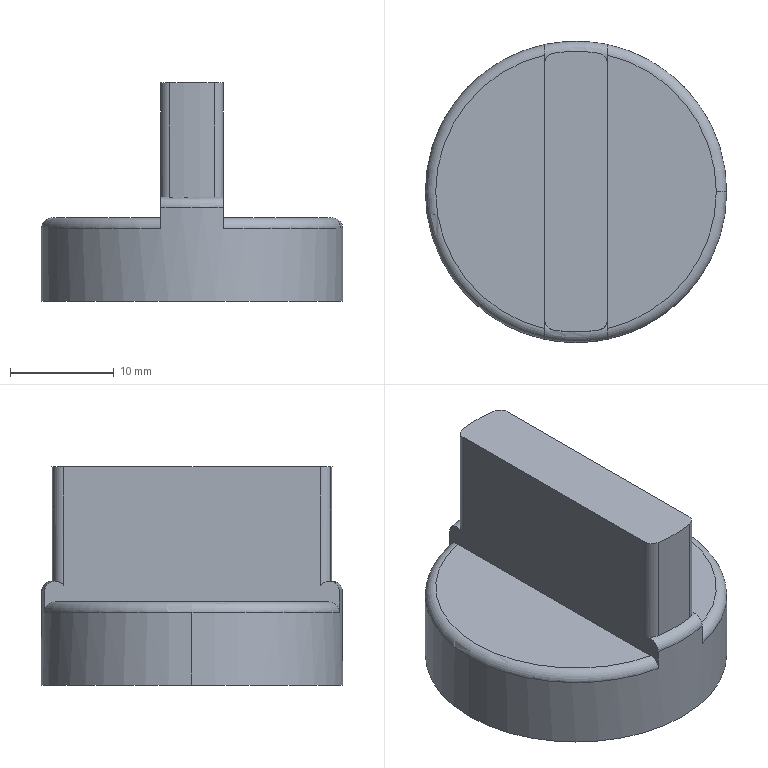Part | STEP file | 7-4-Switch1-619-724_Default | 1 solid | 19 faces | box 29 x 29 x 21 mm | volume 7372 mm3 | cylinder 8 | plane 6 | torus 5 | commonest cylinder face diameters 2 x4 27 x2 29 x2